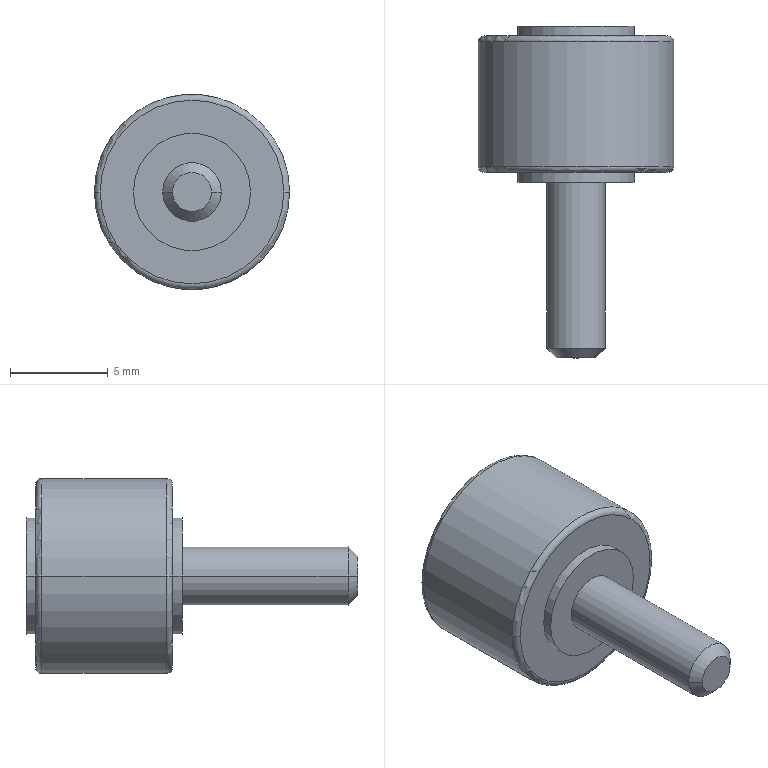Part | NX | 1 solid | 178 faces | box 10 x 17 x 10 mm | volume 639.244 mm3 | plane 164 | cylinder 8 | torus 4 | cone 2 | commonest cylinder face diameters 6 x4 3 x2 10 x2